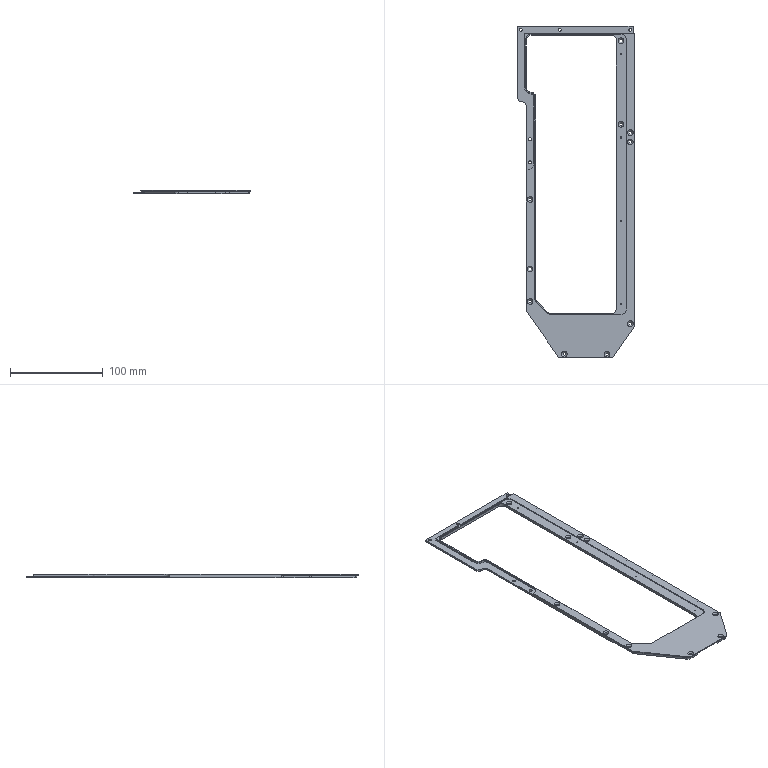NC program | NX | posted with a generic post | part box 127 x 358 x 4 mm
Whole program:
N10 G17 G21 G94 G90
(SPOT_DRILL_COPY_1 , TOOL : CHAMFER_D8-90DEG)
N12 T01 M6
N14 G53
N16 G17 G0 G90 X153.952 Y-40.61 S2500 M3
N18 G43 Z20. H1
N20 G94 G82 G98 Z-2.6 F250. P200 R3.
N22 X103.952 Y-30.61
N24 X48.952
N26 X-6.048
N28 X-61.048
N30 X-111.048
N32 Y28.911
N34 X-61.048
N36 X-6.048
N38 X48.952
N40 X103.952
N42 X153.952
N44 G80
N46 G0 X153.952 Y28.911 Z20.
(PLANAR_MILL_8 , TOOL : CHAMFER_D8-90DEG)
N48 X-190.5 Y-67.5 S3000
N50 Z2.9
N52 G1 Z-0.1 F1000.
N54 X-182.5
N56 X182.5
N58 Y67.5
N60 Y75.5
N62 Z2.9
N64 G0 Z20.
N66 M5
(SPOT_DRILL_COPY_COPY , TOOL : DRILL_D4.3-54-83)
N68 T00 M6
N70 G53
N72 G17 G0 G90 X153.952 Y-40.61 S3000 M3
N74 G43 Z20. H0
N76 G94 G82 G98 Z-15. F200. P200 R3.
N78 X103.952 Y-30.61
N80 X48.952
N82 X-6.048
N84 X-61.048
N86 X-111.048
N88 Y28.911
N90 X-61.048
N92 X-6.048
N94 X48.952
N96 X103.952
N98 X153.952
N100 G80
N102 G0 X153.952 Y28.911 Z20.
N104 M5
(SPOT_DRILL_COPY_COPY_COPY , TOOL : UPPERROW_M5-22-D5.5-60)
N106 M6
N108 G53
N110 G17 G0 G90 X153.952 Y-40.61 S300 M3
N112 G43 Z20. H0
N114 G84 G94 G98 Z-10. F240. R3.
N116 X103.952 Y-30.61
N118 X48.952
N120 X-6.048
N122 X-61.048
N124 X-111.048
N126 Y28.911
N128 X-61.048
N130 X-6.048
N132 X48.952
N134 X103.952
N136 X153.952
N138 G80
N140 G0 X153.952 Y28.911 Z20.
N142 M5
N144 M2